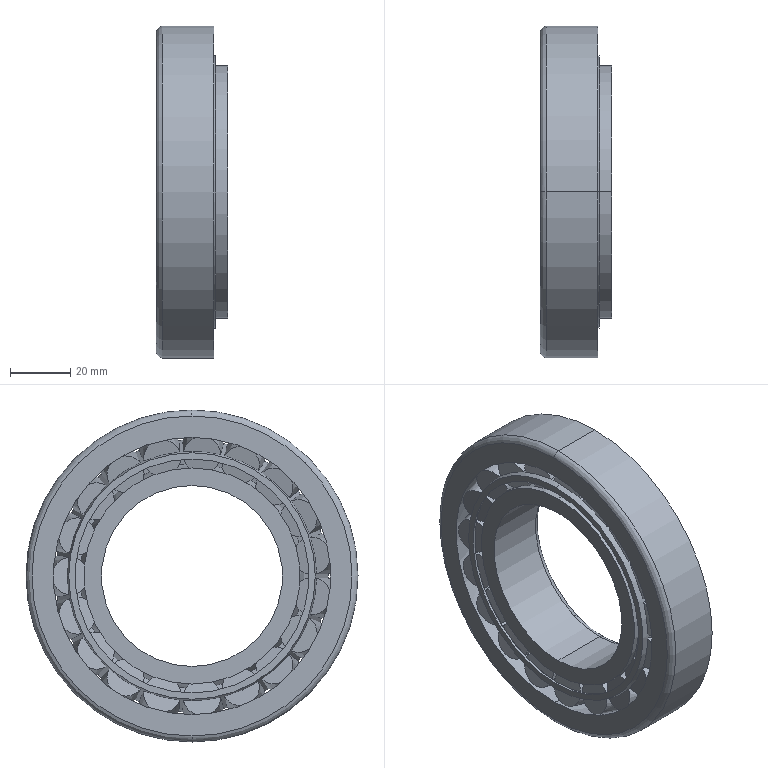Part | STEP file | 30212V11 | 3 solids | 167 faces | box 23.75 x 110 x 110 mm | volume 111845 mm3 | plane 82 | cone 73 | cylinder 8 | torus 4 | commonest cylinder face diameters 60 x2 71.6 x2 83.8 x2 110 x2